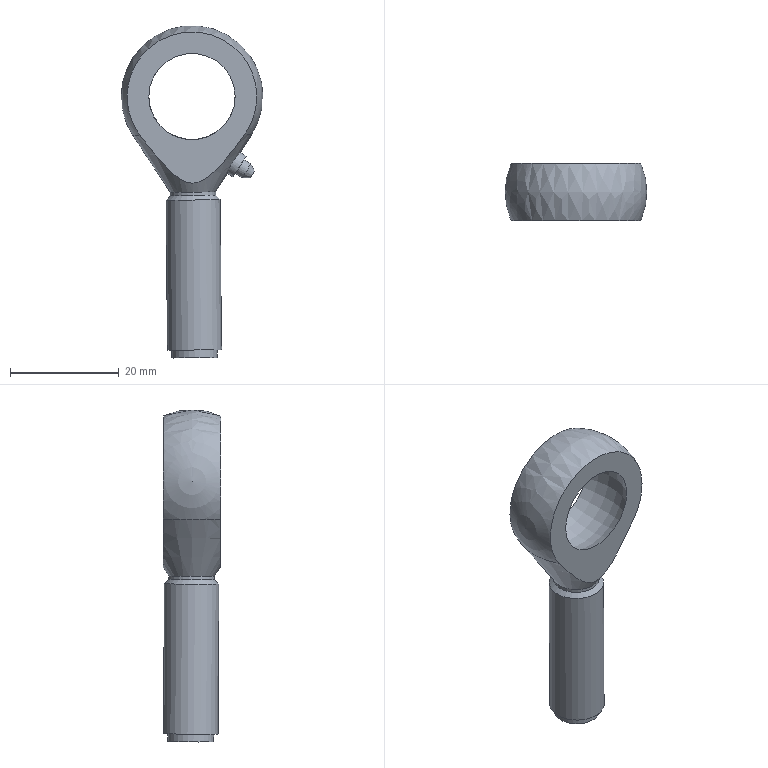Part | NX | features 1 2 | 1 solid | 16 faces | box 26 x 10.639 x 61.044 mm | volume 5586 mm3 | plane 6 | cylinder 5 | cone 3 | torus 1 | sphere 1 | commonest cylinder face diameters 8.376 x2 3 x1 4.5 x1 10 x1
STEP:
#1=CARTESIAN_POINT('',(-103.046,93.069,-231.212));
#2=VERTEX_POINT('',#1);
#3=CARTESIAN_POINT('',(-102.647,93.066,-230.577));
#4=DIRECTION('',(0.8471,0.002225,-0.5315));
#5=DIRECTION('',(-0.5315,0.004511,-0.847));
#6=AXIS2_PLACEMENT_3D('',#3,#4,#5);
#7=CIRCLE('',#6,0.75);
#8=EDGE_CURVE('',#2,#2,#7,.T.);
#9=ORIENTED_EDGE('',*,*,#8,.T.);
#10=EDGE_LOOP('',(#9));
#11=FACE_BOUND('',#10,.T.);
#12=CARTESIAN_POINT('',(-102.448,93.064,-230.259));
#13=DIRECTION('',(0.8471,0.002225,-0.5315));
#14=DIRECTION('',(-0.5315,0.004511,-0.847));
#15=AXIS2_PLACEMENT_3D('',#12,#13,#14);
#16=PLANE('',#15);
#17=ADVANCED_FACE('',(#11),#16,.T.);
#18=ORIENTED_EDGE('',*,*,#8,.F.);
#19=EDGE_LOOP('',(#18));
#20=FACE_BOUND('',#19,.T.);
#21=CARTESIAN_POINT('',(-104.503,93.07,-231.183));
#22=VERTEX_POINT('',#21);
#23=CARTESIAN_POINT('',(-103.706,93.063,-229.913));
#24=DIRECTION('',(0.8471,0.002225,-0.5315));
#25=DIRECTION('',(-0.5315,0.004511,-0.847));
#26=AXIS2_PLACEMENT_3D('',#23,#24,#25);
#27=CIRCLE('',#26,1.5);
#28=EDGE_CURVE('',#22,#22,#27,.T.);
#29=ORIENTED_EDGE('',*,*,#28,.T.);
#30=EDGE_LOOP('',(#29));
#31=FACE_BOUND('',#30,.T.);
#32=CARTESIAN_POINT('',(-102.585,93.066,-230.616));
#33=DIRECTION('',(-0.8471,-0.002225,0.5315));
#34=DIRECTION('',(0.5315,-0.004511,0.847));
#35=AXIS2_PLACEMENT_3D('',#32,#33,#34);
#36=CONICAL_SURFACE('',#35,0.706,0.5404);
#37=ADVANCED_FACE('',(#20,#31),#36,.T.);
#38=CARTESIAN_POINT('',(-104.18,93.053,-227.845));
#39=VERTEX_POINT('',#38);
#40=CARTESIAN_POINT('',(-104.977,93.06,-229.115));
#41=DIRECTION('',(-0.8471,-0.002225,0.5315));
#42=DIRECTION('',(0.5315,-0.004511,0.847));
#43=AXIS2_PLACEMENT_3D('',#40,#41,#42);
#44=CIRCLE('',#43,1.5);
#45=EDGE_CURVE('',#39,#39,#44,.T.);
#46=ORIENTED_EDGE('',*,*,#45,.F.);
#47=EDGE_LOOP('',(#46));
#48=FACE_BOUND('',#47,.T.);
#49=ORIENTED_EDGE('',*,*,#28,.F.);
#50=EDGE_LOOP('',(#49));
#51=FACE_BOUND('',#50,.T.);
#52=CARTESIAN_POINT('',(-104.341,93.062,-229.514));
#53=DIRECTION('',(-0.8471,-0.002225,0.5315));
#54=DIRECTION('',(0.5315,-0.004511,0.847));
#55=AXIS2_PLACEMENT_3D('',#52,#53,#54);
#56=CYLINDRICAL_SURFACE('',#55,1.5);
#57=ADVANCED_FACE('',(#48,#51),#56,.T.);
#58=ORIENTED_EDGE('',*,*,#45,.T.);
#59=EDGE_LOOP('',(#58));
#60=FACE_BOUND('',#59,.T.);
#61=CARTESIAN_POINT('',(-106.173,93.07,-231.021));
#62=VERTEX_POINT('',#61);
#63=CARTESIAN_POINT('',(-104.977,93.06,-229.115));
#64=DIRECTION('',(0.8471,0.002225,-0.5315));
#65=DIRECTION('',(-0.5315,0.004511,-0.847));
#66=AXIS2_PLACEMENT_3D('',#63,#64,#65);
#67=CIRCLE('',#66,2.25);
#68=EDGE_CURVE('',#62,#62,#67,.T.);
#69=ORIENTED_EDGE('',*,*,#68,.T.);
#70=EDGE_LOOP('',(#69));
#71=FACE_BOUND('',#70,.T.);
#72=CARTESIAN_POINT('',(-103.98,93.051,-227.527));
#73=DIRECTION('',(0.8471,0.002225,-0.5315));
#74=DIRECTION('',(-0.5315,0.004511,-0.847));
#75=AXIS2_PLACEMENT_3D('',#72,#73,#74);
#76=PLANE('',#75);
#77=ADVANCED_FACE('',(#60,#71),#76,.T.);
#78=ORIENTED_EDGE('',*,*,#68,.F.);
#79=EDGE_LOOP('',(#78));
#80=FACE_BOUND('',#79,.T.);
#81=CARTESIAN_POINT('',(-104.84,93.047,-226.545));
#82=VERTEX_POINT('',#81);
#83=CARTESIAN_POINT('',(-107.231,93.067,-230.357));
#84=VERTEX_POINT('',#83);
#85=CARTESIAN_POINT('',(-104.84,93.047,-226.545));
#86=CARTESIAN_POINT('',(-104.839,93.639,-226.543));
#87=CARTESIAN_POINT('',(-105.198,94.812,-226.888));
#88=CARTESIAN_POINT('',(-106.335,95.551,-228.251));
#89=CARTESIAN_POINT('',(-107.119,94.823,-229.846));
#90=CARTESIAN_POINT('',(-107.23,93.659,-230.355));
#91=CARTESIAN_POINT('',(-107.231,93.067,-230.357));
#92=B_SPLINE_CURVE_WITH_KNOTS('',3,(#85,#86,#87,#88,#89,#90,#91),.UNSPECIFIED.,.F.,.F.,(4,1,1,1,4),(0.,0.25,0.5,0.75,1.),.UNSPECIFIED.);
#93=EDGE_CURVE('',#82,#84,#92,.T.);
#94=ORIENTED_EDGE('',*,*,#93,.F.);
#95=CARTESIAN_POINT('',(-107.231,93.067,-230.357));
#96=CARTESIAN_POINT('',(-107.231,92.476,-230.361));
#97=CARTESIAN_POINT('',(-107.121,91.306,-229.863));
#98=CARTESIAN_POINT('',(-106.337,90.562,-228.276));
#99=CARTESIAN_POINT('',(-105.2,91.286,-226.906));
#100=CARTESIAN_POINT('',(-104.839,92.455,-226.549));
#101=CARTESIAN_POINT('',(-104.84,93.047,-226.545));
#102=B_SPLINE_CURVE_WITH_KNOTS('',3,(#95,#96,#97,#98,#99,#100,#101),.UNSPECIFIED.,.F.,.F.,(4,1,1,1,4),(0.,0.25,0.5,0.75,1.),.UNSPECIFIED.);
#103=EDGE_CURVE('',#84,#82,#102,.T.);
#104=ORIENTED_EDGE('',*,*,#103,.F.);
#105=EDGE_LOOP('',(#94,#104));
#106=FACE_BOUND('',#105,.T.);
#107=CARTESIAN_POINT('',(-105.93,93.057,-228.518));
#108=DIRECTION('',(-0.8471,-0.002225,0.5315));
#109=DIRECTION('',(0.5315,-0.004511,0.847));
#110=AXIS2_PLACEMENT_3D('',#107,#108,#109);
#111=CYLINDRICAL_SURFACE('',#110,2.25);
#112=ADVANCED_FACE('',(#80,#106),#111,.T.);
#113=CARTESIAN_POINT('',(-105.782,98.245,-216.138));
#114=VERTEX_POINT('',#113);
#115=CARTESIAN_POINT('',(-113.72,98.25,-216.216));
#116=DIRECTION('',(-0.0005134,-1.,-0.005004));
#117=DIRECTION('',(1.,-0.0005629,0.009909));
#118=AXIS2_PLACEMENT_3D('',#115,#116,#117);
#119=CIRCLE('',#118,7.938);
#120=EDGE_CURVE('',#114,#114,#119,.T.);
#121=ORIENTED_EDGE('',*,*,#120,.T.);
#122=EDGE_LOOP('',(#121));
#123=FACE_BOUND('',#122,.T.);
#124=CARTESIAN_POINT('',(-104.049,98.28,-223.139));
#125=VERTEX_POINT('',#124);
#126=CARTESIAN_POINT('',(-123.251,98.29,-223.329));
#127=VERTEX_POINT('',#126);
#128=CARTESIAN_POINT('',(-113.72,98.25,-216.216));
#129=DIRECTION('',(-0.0005134,-1.,-0.005004));
#130=DIRECTION('',(0.8131,0.002495,-0.5821));
#131=AXIS2_PLACEMENT_3D('',#128,#129,#130);
#132=CIRCLE('',#131,11.893);
#133=EDGE_CURVE('',#125,#127,#132,.T.);
#134=ORIENTED_EDGE('',*,*,#133,.F.);
#135=CARTESIAN_POINT('',(-113.562,98.329,-232.11));
#136=VERTEX_POINT('',#135);
#137=CARTESIAN_POINT('',(-113.562,98.329,-232.11));
#138=CARTESIAN_POINT('',(-112.435,98.329,-232.105));
#139=CARTESIAN_POINT('',(-110.408,98.322,-230.913));
#140=CARTESIAN_POINT('',(-108.121,98.308,-228.479));
#141=CARTESIAN_POINT('',(-106.02,98.294,-225.854));
#142=CARTESIAN_POINT('',(-104.701,98.284,-224.049));
#143=CARTESIAN_POINT('',(-104.049,98.28,-223.139));
#144=B_SPLINE_CURVE_WITH_KNOTS('',3,(#137,#138,#139,#140,#141,#142,#143),.UNSPECIFIED.,.F.,.F.,(4,1,1,1,4),(0.,0.25,0.5,0.75,1.),.UNSPECIFIED.);
#145=EDGE_CURVE('',#125,#136,#144,.F.);
#146=ORIENTED_EDGE('',*,*,#145,.T.);
#147=CARTESIAN_POINT('',(-123.251,98.29,-223.329));
#148=CARTESIAN_POINT('',(-122.581,98.295,-224.226));
#149=CARTESIAN_POINT('',(-121.226,98.303,-226.005));
#150=CARTESIAN_POINT('',(-119.074,98.315,-228.588));
#151=CARTESIAN_POINT('',(-116.739,98.325,-230.977));
#152=CARTESIAN_POINT('',(-114.686,98.33,-232.126));
#153=CARTESIAN_POINT('',(-113.562,98.329,-232.11));
#154=B_SPLINE_CURVE_WITH_KNOTS('',3,(#147,#148,#149,#150,#151,#152,#153),.UNSPECIFIED.,.F.,.F.,(4,1,1,1,4),(0.,0.25,0.5,0.75,1.),.UNSPECIFIED.);
#155=EDGE_CURVE('',#136,#127,#154,.F.);
#156=ORIENTED_EDGE('',*,*,#155,.T.);
#157=EDGE_LOOP('',(#134,#146,#156));
#158=FACE_BOUND('',#157,.T.);
#159=CARTESIAN_POINT('',(-139.544,98.352,-234.023));
#160=DIRECTION('',(-0.0005134,-1.,-0.005004));
#161=DIRECTION('',(1.,-0.0005629,0.009909));
#162=AXIS2_PLACEMENT_3D('',#159,#160,#161);
#163=PLANE('',#162);
#164=ADVANCED_FACE('',(#123,#158),#163,.F.);
#165=ORIENTED_EDGE('',*,*,#120,.F.);
#166=EDGE_LOOP('',(#165));
#167=FACE_BOUND('',#166,.T.);
#168=CARTESIAN_POINT('',(-121.663,87.755,-216.348));
#169=VERTEX_POINT('',#168);
#170=CARTESIAN_POINT('',(-113.725,87.75,-216.269));
#171=DIRECTION('',(0.0005134,1.,0.005004));
#172=DIRECTION('',(-1.,0.0005629,-0.009909));
#173=AXIS2_PLACEMENT_3D('',#170,#171,#172);
#174=CIRCLE('',#173,7.938);
#175=EDGE_CURVE('',#169,#169,#174,.T.);
#176=ORIENTED_EDGE('',*,*,#175,.F.);
#177=EDGE_LOOP('',(#176));
#178=FACE_BOUND('',#177,.T.);
#179=CARTESIAN_POINT('',(-113.722,93.,-216.243));
#180=DIRECTION('',(0.0005134,1.,0.005004));
#181=DIRECTION('',(1.,-0.0005629,0.009909));
#182=AXIS2_PLACEMENT_3D('',#179,#180,#181);
#183=DEGENERATE_TOROIDAL_SURFACE('',#182,0.009538,9.525,.F.);
#184=ADVANCED_FACE('',(#167,#178),#183,.T.);
#185=ORIENTED_EDGE('',*,*,#175,.T.);
#186=EDGE_LOOP('',(#185));
#187=FACE_BOUND('',#186,.T.);
#188=CARTESIAN_POINT('',(-123.256,87.791,-223.382));
#189=VERTEX_POINT('',#188);
#190=CARTESIAN_POINT('',(-104.055,87.78,-223.192));
#191=VERTEX_POINT('',#190);
#192=CARTESIAN_POINT('',(-113.725,87.75,-216.269));
#193=DIRECTION('',(0.0005134,1.,0.005004));
#194=DIRECTION('',(-0.8014,0.003404,-0.5981));
#195=AXIS2_PLACEMENT_3D('',#192,#193,#194);
#196=CIRCLE('',#195,11.893);
#197=EDGE_CURVE('',#189,#191,#196,.T.);
#198=ORIENTED_EDGE('',*,*,#197,.F.);
#199=CARTESIAN_POINT('',(-113.567,87.83,-232.162));
#200=VERTEX_POINT('',#199);
#201=CARTESIAN_POINT('',(-113.567,87.83,-232.162));
#202=CARTESIAN_POINT('',(-114.695,87.83,-232.18));
#203=CARTESIAN_POINT('',(-116.744,87.825,-231.029));
#204=CARTESIAN_POINT('',(-119.08,87.815,-228.64));
#205=CARTESIAN_POINT('',(-121.232,87.803,-226.057));
#206=CARTESIAN_POINT('',(-122.587,87.795,-224.278));
#207=CARTESIAN_POINT('',(-123.256,87.791,-223.382));
#208=B_SPLINE_CURVE_WITH_KNOTS('',3,(#201,#202,#203,#204,#205,#206,#207),.UNSPECIFIED.,.F.,.F.,(4,1,1,1,4),(0.,0.25,0.5,0.75,1.),.UNSPECIFIED.);
#209=EDGE_CURVE('',#200,#189,#208,.T.);
#210=ORIENTED_EDGE('',*,*,#209,.F.);
#211=CARTESIAN_POINT('',(-104.055,87.78,-223.192));
#212=CARTESIAN_POINT('',(-104.706,87.785,-224.101));
#213=CARTESIAN_POINT('',(-106.026,87.794,-225.907));
#214=CARTESIAN_POINT('',(-108.127,87.809,-228.532));
#215=CARTESIAN_POINT('',(-110.413,87.822,-230.967));
#216=CARTESIAN_POINT('',(-112.443,87.829,-232.156));
#217=CARTESIAN_POINT('',(-113.567,87.83,-232.162));
#218=B_SPLINE_CURVE_WITH_KNOTS('',3,(#211,#212,#213,#214,#215,#216,#217),.UNSPECIFIED.,.F.,.F.,(4,1,1,1,4),(0.,0.25,0.5,0.75,1.),.UNSPECIFIED.);
#219=EDGE_CURVE('',#191,#200,#218,.T.);
#220=ORIENTED_EDGE('',*,*,#219,.F.);
#221=EDGE_LOOP('',(#198,#210,#220));
#222=FACE_BOUND('',#221,.T.);
#223=CARTESIAN_POINT('',(-139.853,87.7,-203.527));
#224=DIRECTION('',(0.0005134,1.,0.005004));
#225=DIRECTION('',(-1.,0.0005629,-0.009909));
#226=AXIS2_PLACEMENT_3D('',#223,#224,#225);
#227=PLANE('',#226);
#228=ADVANCED_FACE('',(#187,#222),#227,.F.);
#229=CARTESIAN_POINT('',(-113.249,89.052,-264.261));
#230=VERTEX_POINT('',#229);
#231=CARTESIAN_POINT('',(-113.247,93.24,-264.24));
#232=DIRECTION('',(0.009912,0.004999,-0.9999));
#233=DIRECTION('',(-0.0005134,-1.,-0.005004));
#234=AXIS2_PLACEMENT_3D('',#231,#232,#233);
#235=CIRCLE('',#234,4.188);
#236=EDGE_CURVE('',#230,#230,#235,.T.);
#237=ORIENTED_EDGE('',*,*,#236,.T.);
#238=EDGE_LOOP('',(#237));
#239=FACE_BOUND('',#238,.T.);
#240=CARTESIAN_POINT('',(-111.153,93.239,-264.219));
#241=DIRECTION('',(0.009912,0.004999,-0.9999));
#242=DIRECTION('',(-0.0005134,-1.,-0.005004));
#243=AXIS2_PLACEMENT_3D('',#240,#241,#242);
#244=PLANE('',#243);
#245=ADVANCED_FACE('',(#239),#244,.T.);
#246=ORIENTED_EDGE('',*,*,#236,.F.);
#247=EDGE_LOOP('',(#246));
#248=FACE_BOUND('',#247,.T.);
#249=CARTESIAN_POINT('',(-113.259,97.421,-262.769));
#250=VERTEX_POINT('',#249);
#251=CARTESIAN_POINT('',(-113.261,93.233,-262.79));
#252=DIRECTION('',(-0.009912,-0.004999,0.9999));
#253=DIRECTION('',(0.0005134,1.,0.005004));
#254=AXIS2_PLACEMENT_3D('',#251,#252,#253);
#255=CIRCLE('',#254,4.188);
#256=EDGE_CURVE('',#250,#250,#255,.T.);
#257=ORIENTED_EDGE('',*,*,#256,.F.);
#258=EDGE_LOOP('',(#257));
#259=FACE_BOUND('',#258,.T.);
#260=CARTESIAN_POINT('',(-113.254,93.236,-263.515));
#261=DIRECTION('',(-0.009912,-0.004999,0.9999));
#262=DIRECTION('',(0.0005134,1.,0.005004));
#263=AXIS2_PLACEMENT_3D('',#260,#261,#262);
#264=CYLINDRICAL_SURFACE('',#263,4.188);
#265=ADVANCED_FACE('',(#248,#259),#264,.T.);
#266=ORIENTED_EDGE('',*,*,#256,.T.);
#267=EDGE_LOOP('',(#266));
#268=FACE_BOUND('',#267,.T.);
#269=CARTESIAN_POINT('',(-113.258,98.233,-262.765));
#270=VERTEX_POINT('',#269);
#271=CARTESIAN_POINT('',(-113.261,93.233,-262.79));
#272=DIRECTION('',(0.009912,0.004999,-0.9999));
#273=DIRECTION('',(0.0005134,1.,0.005004));
#274=AXIS2_PLACEMENT_3D('',#271,#272,#273);
#275=CIRCLE('',#274,5.);
#276=EDGE_CURVE('',#270,#270,#275,.T.);
#277=ORIENTED_EDGE('',*,*,#276,.T.);
#278=EDGE_LOOP('',(#277));
#279=FACE_BOUND('',#278,.T.);
#280=CARTESIAN_POINT('',(-108.667,93.23,-262.744));
#281=DIRECTION('',(0.009912,0.004999,-0.9999));
#282=DIRECTION('',(-0.0005134,-1.,-0.005004));
#283=AXIS2_PLACEMENT_3D('',#280,#281,#282);
#284=PLANE('',#283);
#285=ADVANCED_FACE('',(#268,#279),#284,.T.);
#286=CARTESIAN_POINT('',(-113.531,98.095,-235.216));
#287=VERTEX_POINT('',#286);
#288=CARTESIAN_POINT('',(-113.534,93.095,-235.241));
#289=DIRECTION('',(-0.009912,-0.004999,0.9999));
#290=DIRECTION('',(0.0005134,1.,0.005004));
#291=AXIS2_PLACEMENT_3D('',#288,#289,#290);
#292=CIRCLE('',#291,5.);
#293=EDGE_CURVE('',#287,#287,#292,.T.);
#294=ORIENTED_EDGE('',*,*,#293,.F.);
#295=EDGE_LOOP('',(#294));
#296=FACE_BOUND('',#295,.T.);
#297=ORIENTED_EDGE('',*,*,#276,.F.);
#298=EDGE_LOOP('',(#297));
#299=FACE_BOUND('',#298,.T.);
#300=CARTESIAN_POINT('',(-113.397,93.164,-249.016));
#301=DIRECTION('',(-0.009912,-0.004999,0.9999));
#302=DIRECTION('',(0.0005134,1.,0.005004));
#303=AXIS2_PLACEMENT_3D('',#300,#301,#302);
#304=CYLINDRICAL_SURFACE('',#303,5.);
#305=ADVANCED_FACE('',(#296,#299),#304,.T.);
#306=ORIENTED_EDGE('',*,*,#293,.T.);
#307=EDGE_LOOP('',(#306));
#308=FACE_BOUND('',#307,.T.);
#309=CARTESIAN_POINT('',(-113.544,88.903,-234.451));
#310=VERTEX_POINT('',#309);
#311=CARTESIAN_POINT('',(-113.542,93.091,-234.43));
#312=DIRECTION('',(0.009912,0.004999,-0.9999));
#313=DIRECTION('',(-0.0005134,-1.,-0.005004));
#314=AXIS2_PLACEMENT_3D('',#311,#312,#313);
#315=CIRCLE('',#314,4.188);
#316=EDGE_CURVE('',#310,#310,#315,.T.);
#317=ORIENTED_EDGE('',*,*,#316,.T.);
#318=EDGE_LOOP('',(#317));
#319=FACE_BOUND('',#318,.T.);
#320=CARTESIAN_POINT('',(-113.543,93.091,-234.369));
#321=DIRECTION('',(0.009912,0.004999,-0.9999));
#322=DIRECTION('',(-0.0005134,-1.,-0.005004));
#323=AXIS2_PLACEMENT_3D('',#320,#321,#322);
#324=CONICAL_SURFACE('',#323,4.128,0.7854);
#325=ADVANCED_FACE('',(#308,#319),#324,.T.);
#326=CARTESIAN_POINT('',(-113.546,97.276,-233.771));
#327=VERTEX_POINT('',#326);
#328=CARTESIAN_POINT('',(-113.548,93.088,-233.792));
#329=DIRECTION('',(-0.009912,-0.004999,0.9999));
#330=DIRECTION('',(0.0005134,1.,0.005004));
#331=AXIS2_PLACEMENT_3D('',#328,#329,#330);
#332=CIRCLE('',#331,4.188);
#333=EDGE_CURVE('',#327,#327,#332,.T.);
#334=ORIENTED_EDGE('',*,*,#333,.F.);
#335=EDGE_LOOP('',(#334));
#336=FACE_BOUND('',#335,.T.);
#337=ORIENTED_EDGE('',*,*,#316,.F.);
#338=EDGE_LOOP('',(#337));
#339=FACE_BOUND('',#338,.T.);
#340=CARTESIAN_POINT('',(-113.545,93.089,-234.111));
#341=DIRECTION('',(-0.009912,-0.004999,0.9999));
#342=DIRECTION('',(0.0005134,1.,0.005004));
#343=AXIS2_PLACEMENT_3D('',#340,#341,#342);
#344=CYLINDRICAL_SURFACE('',#343,4.188);
#345=ADVANCED_FACE('',(#336,#339),#344,.T.);
#346=ORIENTED_EDGE('',*,*,#333,.T.);
#347=EDGE_LOOP('',(#346));
#348=FACE_BOUND('',#347,.T.);
#349=ORIENTED_EDGE('',*,*,#155,.F.);
#350=ORIENTED_EDGE('',*,*,#145,.F.);
#351=CARTESIAN_POINT('',(-113.653,93.035,-223.261));
#352=DIRECTION('',(-0.009912,-0.004999,0.9999));
#353=DIRECTION('',(0.8771,-0.4803,0.006293));
#354=AXIS2_PLACEMENT_3D('',#351,#352,#353);
#355=CIRCLE('',#354,10.943);
#356=EDGE_CURVE('',#191,#125,#355,.T.);
#357=ORIENTED_EDGE('',*,*,#356,.F.);
#358=ORIENTED_EDGE('',*,*,#219,.T.);
#359=ORIENTED_EDGE('',*,*,#209,.T.);
#360=CARTESIAN_POINT('',(-113.653,93.035,-223.261));
#361=DIRECTION('',(-0.009912,-0.004999,0.9999));
#362=DIRECTION('',(-1.,0.0005629,-0.009909));
#363=AXIS2_PLACEMENT_3D('',#360,#361,#362);
#364=CIRCLE('',#363,10.943);
#365=EDGE_CURVE('',#127,#189,#364,.T.);
#366=ORIENTED_EDGE('',*,*,#365,.F.);
#367=EDGE_LOOP('',(#349,#350,#357,#358,#359,#366));
#368=FACE_BOUND('',#367,.T.);
#369=ORIENTED_EDGE('',*,*,#103,.T.);
#370=ORIENTED_EDGE('',*,*,#93,.T.);
#371=EDGE_LOOP('',(#369,#370));
#372=FACE_BOUND('',#371,.T.);
#373=CARTESIAN_POINT('',(-113.546,93.089,-234.002));
#374=DIRECTION('',(-0.009912,-0.004999,0.9999));
#375=DIRECTION('',(0.0005134,1.,0.005004));
#376=AXIS2_PLACEMENT_3D('',#373,#374,#375);
#377=CONICAL_SURFACE('',#376,4.053,0.5703);
#378=ADVANCED_FACE('',(#348,#368,#372),#377,.T.);
#379=ORIENTED_EDGE('',*,*,#356,.T.);
#380=ORIENTED_EDGE('',*,*,#133,.T.);
#381=ORIENTED_EDGE('',*,*,#365,.T.);
#382=ORIENTED_EDGE('',*,*,#197,.T.);
#383=EDGE_LOOP('',(#379,#380,#381,#382));
#384=FACE_BOUND('',#383,.T.);
#385=CARTESIAN_POINT('',(-113.722,93.,-216.243));
#386=DIRECTION('',(1.,-0.0005629,0.009909));
#387=DIRECTION('',(0.009912,0.004999,-0.9999));
#388=AXIS2_PLACEMENT_3D('',#385,#386,#387);
#389=SPHERICAL_SURFACE('',#388,13.);
#390=ADVANCED_FACE('',(#384),#389,.T.);
#391=CLOSED_SHELL('',(#17,#37,#57,#77,#112,#164,#184,#228,#245,#265,#285,#305,#325,#345,#378,#390));
#392=MANIFOLD_SOLID_BREP('',#391);
#393=(LENGTH_UNIT()NAMED_UNIT(*)SI_UNIT(.MILLI.,.METRE.));
#394=UNCERTAINTY_MEASURE_WITH_UNIT(LENGTH_MEASURE(0.0508),#393,'','');
#395=(NAMED_UNIT(*)PLANE_ANGLE_UNIT()SI_UNIT($,.RADIAN.));
#396=(NAMED_UNIT(*)SI_UNIT($,.STERADIAN.)SOLID_ANGLE_UNIT());
#397=(GEOMETRIC_REPRESENTATION_CONTEXT(3)GLOBAL_UNCERTAINTY_ASSIGNED_CONTEXT((#394))GLOBAL_UNIT_ASSIGNED_CONTEXT((#393,#395,#396))REPRESENTATION_CONTEXT('',''));
#398=ADVANCED_BREP_SHAPE_REPRESENTATION('',(#392),#397);